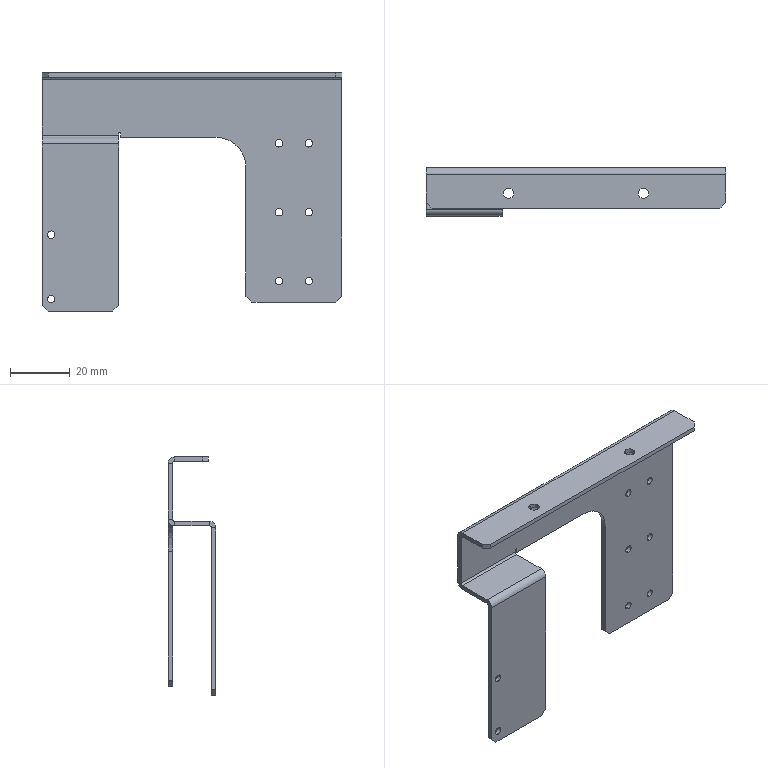Part | SolidWorks | features EdgeFlange 3, HoleWzd 3, Chamfer 1, Fillet 1, FlatPattern 1, ICE 1, LPattern 1, SMBaseFlange 1, SheetMetal 1 | 1 solid | 63 faces | box 100 x 16 x 79.5 mm | volume 10218 mm3 | plane 36 | cylinder 27 | commonest cylinder face diameters 2.5 x16 3.5 x4 1.473 x3 4.473 x3 20 x1